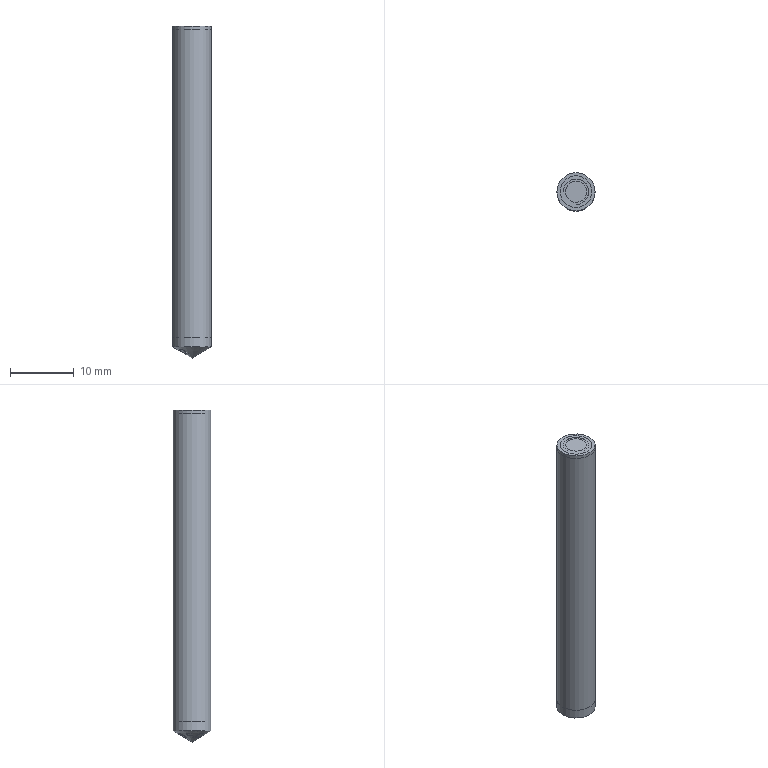Part | STEP file | EE030605000 | 2 solids | 45 faces | box 6 x 6 x 52.232 mm | volume 2767 mm3 | plane 15 | other 13 | cone 11 | cylinder 5 | torus 1 | commonest cylinder face diameters 6 x2 3.333 x1 3.987 x1 4 x1